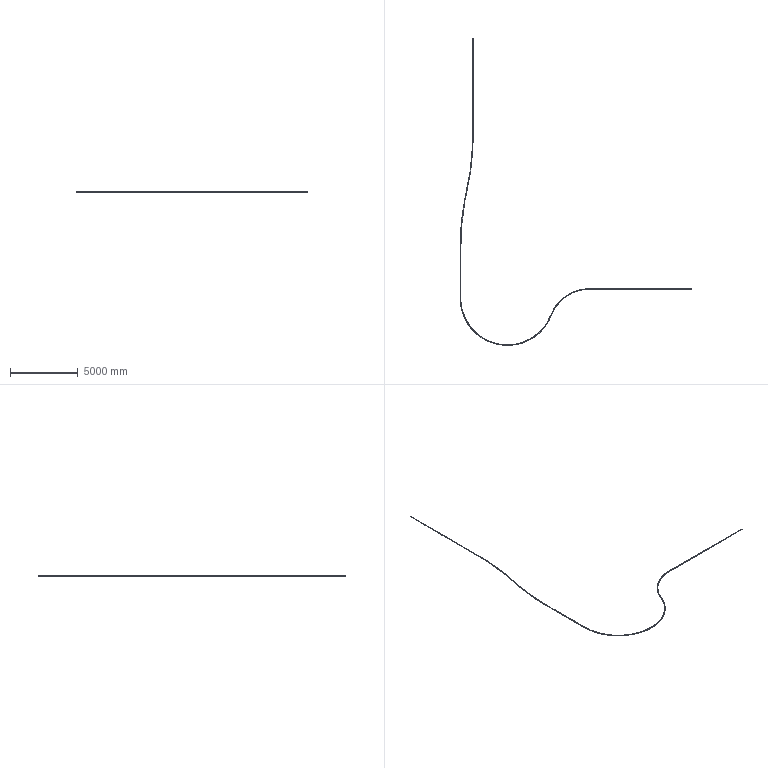Part | SolidWorks | features Sweep 1 | 1 solid | 22 faces | box 17149 x 22725 x 30 mm | volume 6973781 mm3 | spline 14 | plane 8